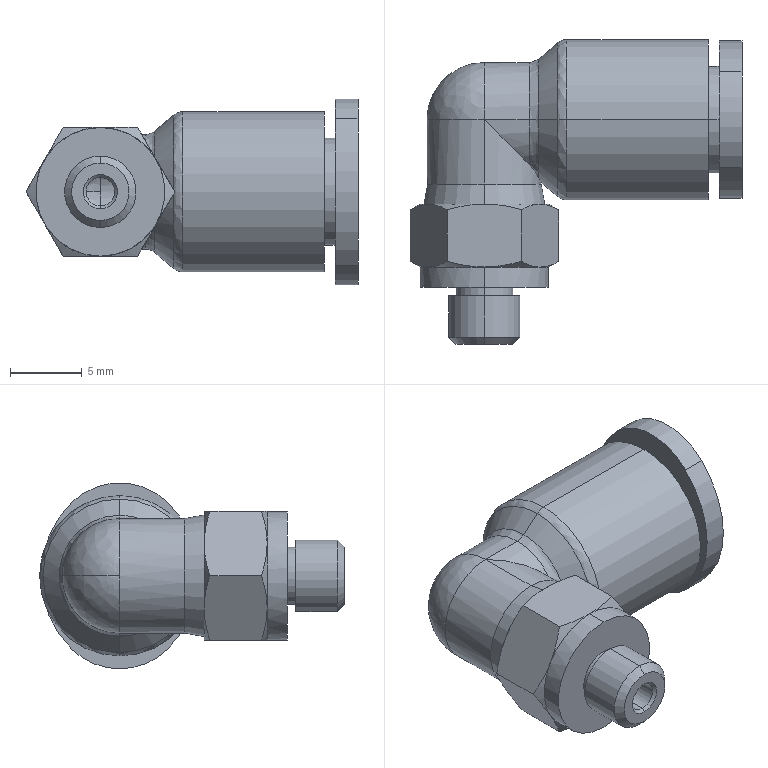Part | STEP file | 0246_013_MSELL6-M5 | 1 solid | 72 faces | box 23.196 x 21.3 x 13 mm | volume 1676 mm3 | cylinder 28 | cone 20 | plane 15 | spline 9 | commonest cylinder face diameters 4 x6 8 x5 9.558 x3 2 x2 5 x2 6 x2